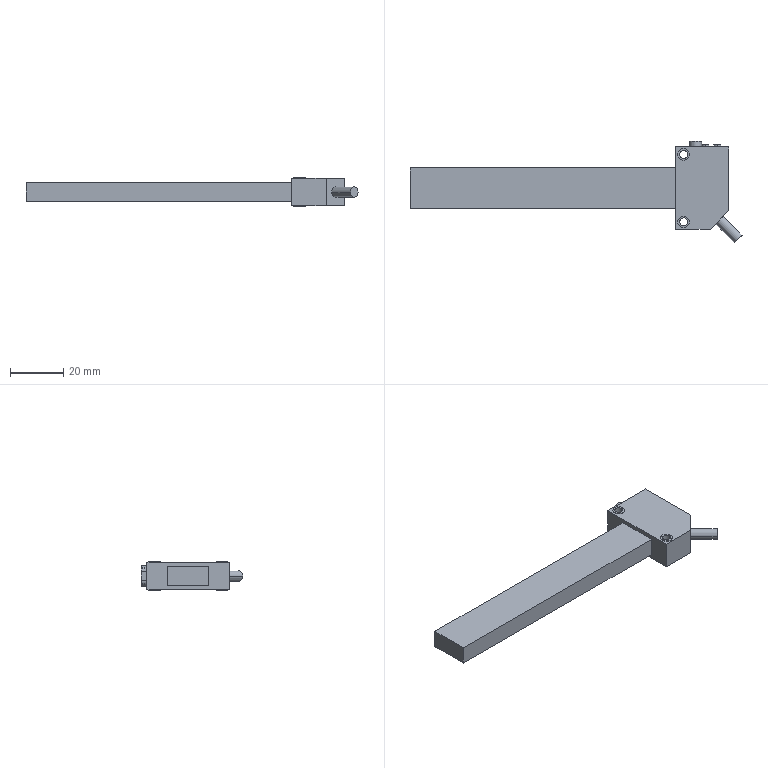Part | STEP file | E3Z_D61-2M^Material sensor assembly | 1 solid | 68 faces | box 124.985 x 38.085 x 10.8 mm | volume 16884 mm3 | plane 47 | cylinder 21 | commonest cylinder face diameters 4.4 x8 2.6 x4 3 x4 4.5 x3 4 x2